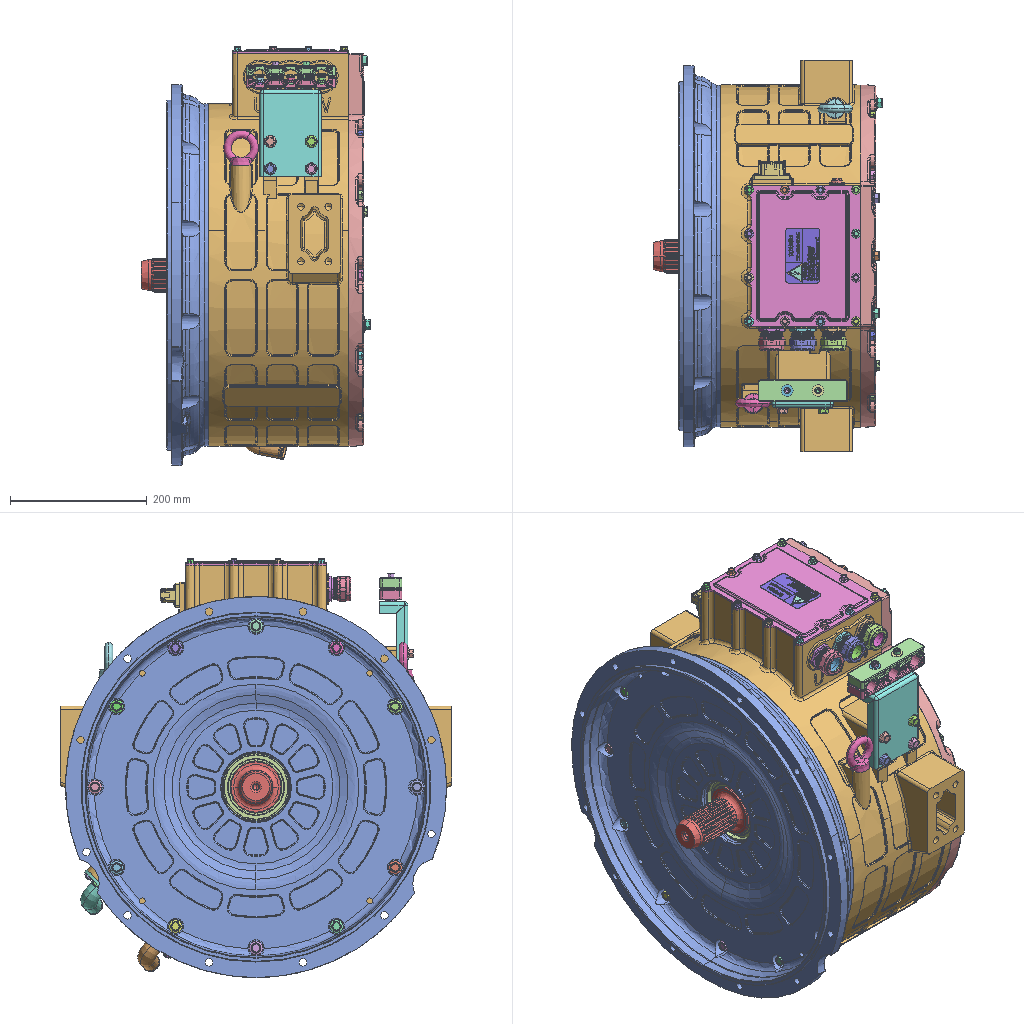Assembly | SolidWorks | 132 different items | 132 placed | box 335 x 572 x 612 mm
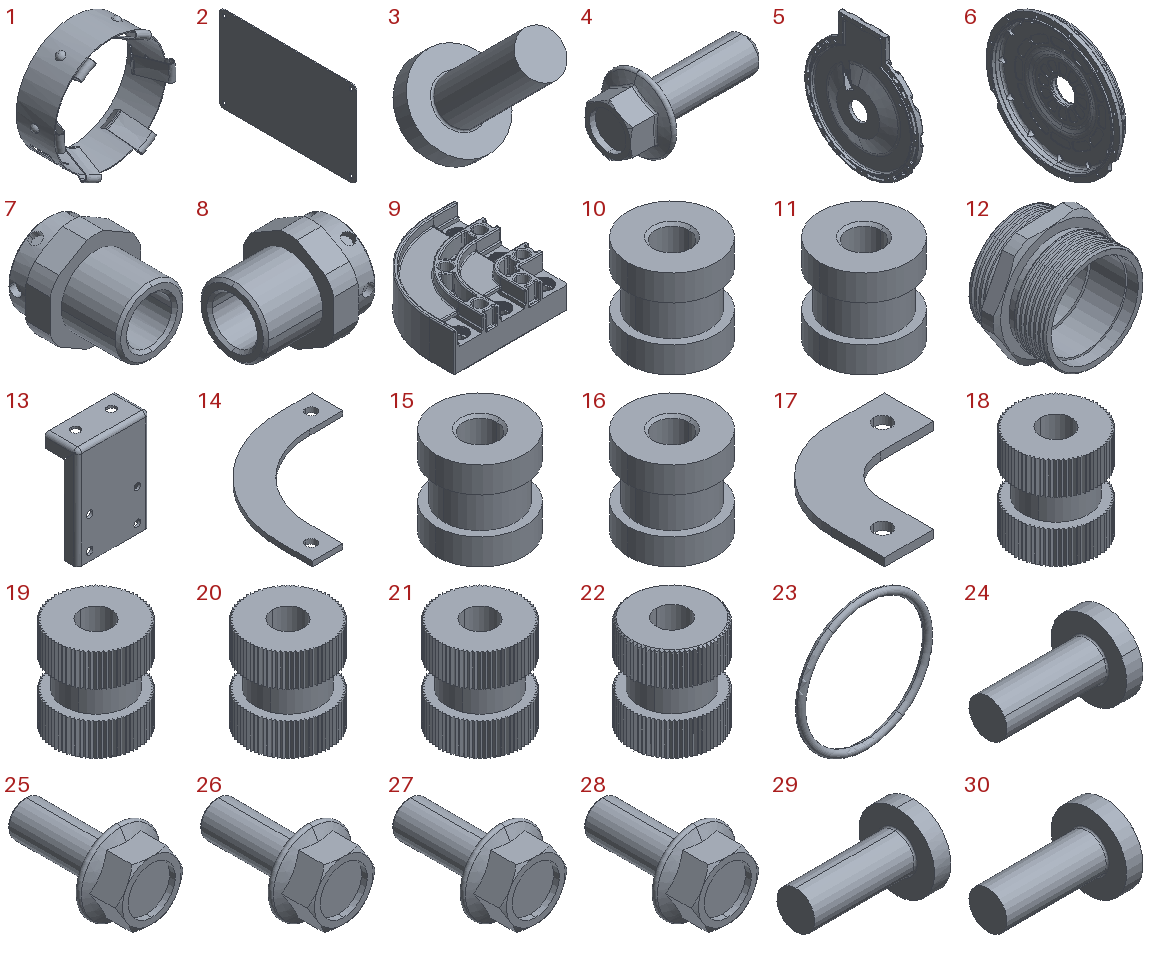Parts list (item | quantity | size | volume | features):
1 | x1 | 28 x 11 x 26.6 mm | 215.957 mm3 | features BaseBody 1
2 | x1 | - | 3306 mm3 | features BaseBody 1
3 | x1 | 12 x 19.516 x 19.516 mm | 825.398 mm3 | features BaseBody 1
4 | x1 | 39.7 x 20.8 x 20.8 mm | 3844 mm3 | features BaseBody 1
5 | x1 | 38.5 x 500 x 573.5 mm | 2957583 mm3 | features BaseBody 1
6 | x1 | 70 x 556.6 x 556.6 mm | 4634291 mm3 | features BaseBody 1
7 | x1 | 16 x 18.5 x 17 mm | 1862 mm3 | features BaseBody 1
8 | x1 | 18.5 x 16 x 17 mm | 1862 mm3 | features BaseBody 1
9 | x1 | 120 x 120 x 40 mm | 221994 mm3 | features BaseBody 1
10 | x1 | 17 x 17 x 17 mm | 2778 mm3 | features BaseBody 1
11 | x1 | 17 x 17 x 17 mm | 2778 mm3 | features BaseBody 1
12 | x1 | 39 x 25 x 36.772 mm | 7027 mm3 | features BaseBody 1
13 | x1 | 90 x 41 x 127.2 mm | 53821 mm3 | features BaseBody 1
14 | x1 | 115 x 115 x 4 mm | 16149 mm3 | features BaseBody 1
15 | x1 | 17 x 17 x 17 mm | 2778 mm3 | features BaseBody 1
16 | x1 | 17 x 17 x 17 mm | 2778 mm3 | features BaseBody 1
17 | x1 | 70 x 70 x 4 mm | 9364 mm3 | features BaseBody 1
18 | x1 | 18.005 x 18.005 x 20 mm | 3580 mm3 | features BaseBody 1
19 | x1 | 18.005 x 18.005 x 20 mm | 3580 mm3 | features BaseBody 1
20 | x1 | 18.005 x 18.005 x 20 mm | 3580 mm3 | features BaseBody 1
21 | x1 | 18.005 x 18.005 x 20 mm | 3580 mm3 | features BaseBody 1
22 | x1 | 18.005 x 18.005 x 20 mm | 3583 mm3 | features BaseBody 1
23 | x1 | 33.8 x 1.8 x 33.8 mm | 255.82 mm3 | features BaseBody 1
24 | x1 | 20.395 x 12 x 12 mm | 825.398 mm3 | features BaseBody 1
25 | x1 | 18 x 28.1 x 18 mm | 2194 mm3 | features BaseBody 1
26 | x1 | 18 x 28.1 x 18 mm | 2194 mm3 | features BaseBody 1
27 | x1 | 18 x 28.1 x 18 mm | 2194 mm3 | features BaseBody 1
28 | x1 | 18 x 28.1 x 18 mm | 2194 mm3 | features BaseBody 1
29 | x1 | 20.395 x 12 x 12 mm | 825.398 mm3 | features BaseBody 1
30 | x1 | 20.395 x 12 x 12 mm | 825.398 mm3 | features BaseBody 1
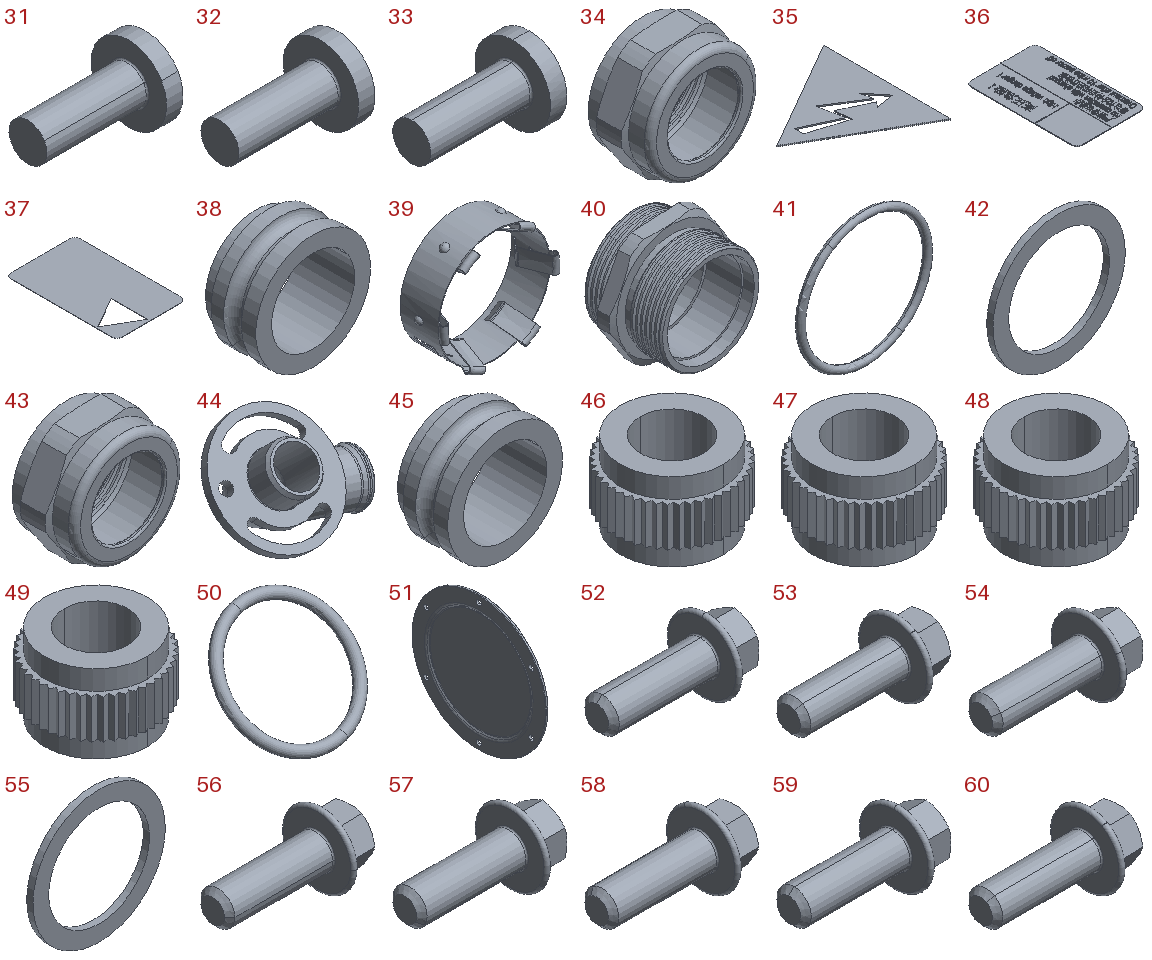31 | x1 | 20.395 x 12 x 12 mm | 825.398 mm3 | features BaseBody 1
32 | x1 | 20.395 x 12 x 12 mm | 825.398 mm3 | features BaseBody 1
33 | x1 | 20.395 x 12 x 12 mm | 825.398 mm3 | features BaseBody 1
34 | x1 | 39 x 20 x 36.772 mm | 4794 mm3 | features BaseBody 1
35 | x1 | 18.841 x 21.756 x 0.2 mm | 36.989 mm3 | features BaseBody 1
36 | x1 | 50 x 80 x 0.7 mm | 2057 mm3 | features BaseBody 1
37 | x1 | 50 x 80 x 0.2 mm | 739.101 mm3 | features BaseBody 1
38 | x1 | 32 x 16 x 32 mm | 4523 mm3 | features BaseBody 1
39 | x1 | 28 x 11 x 26.6 mm | 215.957 mm3 | features BaseBody 1
40 | x1 | 39 x 25 x 36.772 mm | 7027 mm3 | features BaseBody 1
41 | x1 | 33.8 x 1.8 x 33.8 mm | 255.82 mm3 | features BaseBody 1
42 | x1 | 31.8 x 1.5 x 31.8 mm | 501.398 mm3 | features BaseBody 1
43 | x1 | 39 x 20 x 36.772 mm | 4794 mm3 | features BaseBody 1
44 | x1 | 86.222 x 51.732 x 65.283 mm | 24499 mm3 | features BaseBody 1
45 | x1 | 32 x 16 x 32 mm | 4523 mm3 | features BaseBody 1
46 | x1 | 11.993 x 11.985 x 8 mm | 502.783 mm3 | features BaseBody 1
47 | x1 | 11.993 x 11.985 x 8 mm | 502.783 mm3 | features BaseBody 1
48 | x1 | 11.993 x 11.985 x 8 mm | 502.783 mm3 | features BaseBody 1
49 | x1 | 11.993 x 11.985 x 8 mm | 502.783 mm3 | features BaseBody 1
50 | x1 | 32.65 x 23.863 x 23.863 mm | 519.82 mm3 | features BaseBody 1
51 | x1 | 5 x 166 x 166 mm | 64748 mm3 | features BaseBody 1
52 | x1 | 39.7 x 20.8 x 20.8 mm | 3844 mm3 | features BaseBody 1
53 | x1 | 39.7 x 20.8 x 20.8 mm | 3844 mm3 | features BaseBody 1
54 | x1 | 39.7 x 20.8 x 20.8 mm | 3844 mm3 | features BaseBody 1
55 | x1 | 31.8 x 1.5 x 31.8 mm | 501.398 mm3 | features BaseBody 1
56 | x1 | 39.7 x 20.8 x 20.8 mm | 3844 mm3 | features BaseBody 1
57 | x1 | 39.7 x 20.8 x 20.8 mm | 3844 mm3 | features BaseBody 1
58 | x1 | 39.7 x 20.8 x 20.8 mm | 3844 mm3 | features BaseBody 1
59 | x1 | 39.7 x 20.8 x 20.8 mm | 3844 mm3 | features BaseBody 1
60 | x1 | 39.7 x 20.8 x 20.8 mm | 3844 mm3 | features BaseBody 1
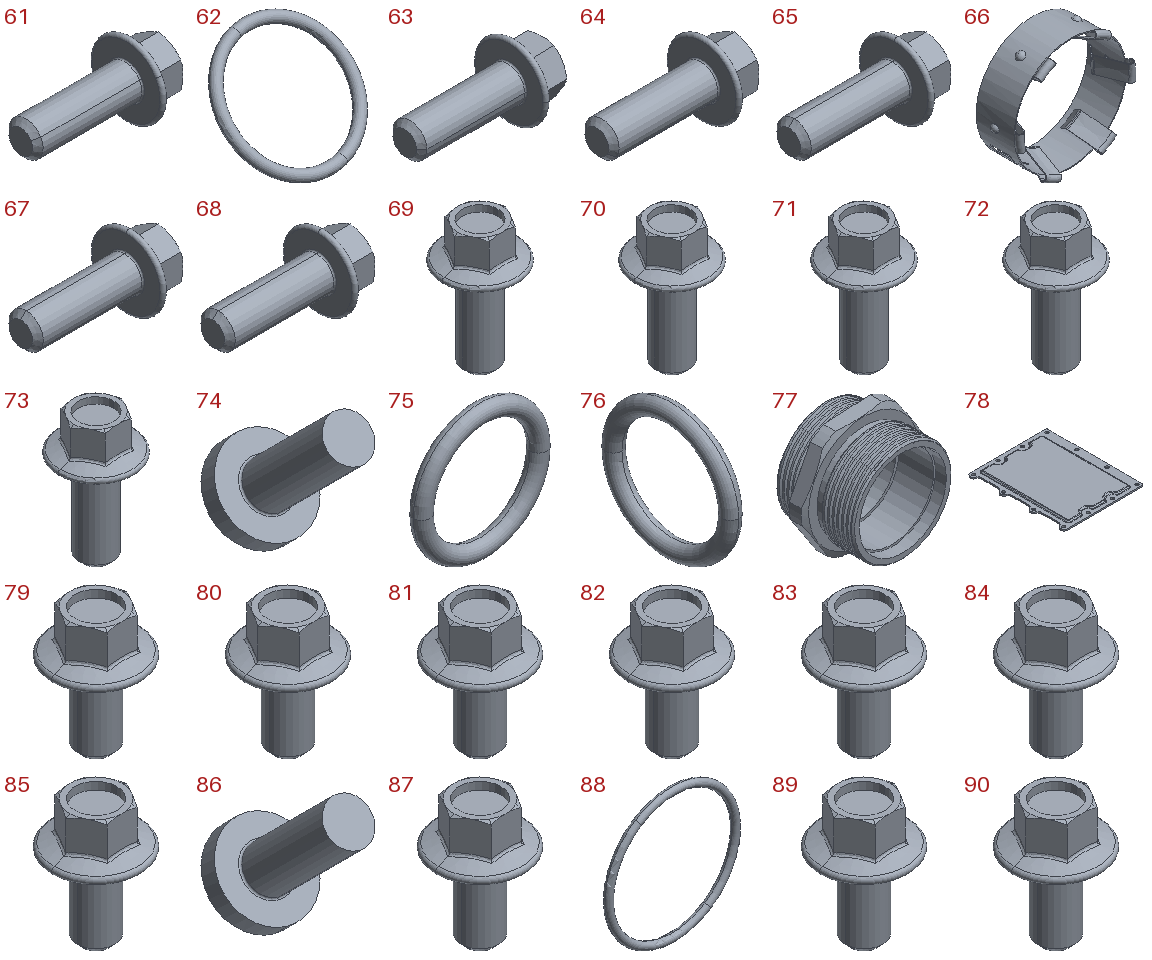61 | x1 | 39.7 x 20.8 x 20.8 mm | 3844 mm3 | features BaseBody 1
62 | x1 | 32.65 x 23.863 x 23.863 mm | 519.82 mm3 | features BaseBody 1
63 | x1 | 39.7 x 20.8 x 20.8 mm | 3844 mm3 | features BaseBody 1
64 | x1 | 39.7 x 20.8 x 20.8 mm | 3844 mm3 | features BaseBody 1
65 | x1 | 39.7 x 20.8 x 20.8 mm | 3844 mm3 | features BaseBody 1
66 | x1 | 28 x 11 x 26.6 mm | 215.957 mm3 | features BaseBody 1
67 | x1 | 39.7 x 20.8 x 20.8 mm | 3844 mm3 | features BaseBody 1
68 | x1 | 39.7 x 20.8 x 20.8 mm | 3844 mm3 | features BaseBody 1
69 | x1 | 17 x 17 x 28.5 mm | 1813 mm3 | features BaseBody 1
70 | x1 | 17 x 17 x 28.5 mm | 1813 mm3 | features BaseBody 1
71 | x1 | 17 x 17 x 28.5 mm | 1813 mm3 | features BaseBody 1
72 | x1 | 17 x 17 x 28.5 mm | 1813 mm3 | features BaseBody 1
73 | x1 | 17 x 17 x 28.5 mm | 1813 mm3 | features BaseBody 1
74 | x1 | 12 x 19.516 x 19.516 mm | 825.398 mm3 | features BaseBody 1
75 | x1 | 16 x 2 x 16 mm | 138.174 mm3 | features BaseBody 1
76 | x1 | 2 x 16 x 16 mm | 138.174 mm3 | features BaseBody 1
77 | x1 | 39 x 25 x 36.772 mm | 7027 mm3 | features BaseBody 1
78 | x1 | 170 x 206 x 6 mm | 103348 mm3 | features BaseBody 1
79 | x1 | 13.6 x 13.6 x 18.9 mm | 775.835 mm3 | features BaseBody 1
80 | x1 | 13.6 x 13.6 x 18.9 mm | 775.834 mm3 | features BaseBody 1
81 | x1 | 13.6 x 13.6 x 18.9 mm | 775.835 mm3 | features BaseBody 1
82 | x1 | 13.6 x 13.6 x 18.9 mm | 775.835 mm3 | features BaseBody 1
83 | x1 | 13.6 x 13.6 x 18.9 mm | 775.835 mm3 | features BaseBody 1
84 | x1 | 13.6 x 13.6 x 18.9 mm | 775.835 mm3 | features BaseBody 1
85 | x1 | 13.6 x 13.6 x 18.9 mm | 775.835 mm3 | features BaseBody 1
86 | x1 | 12 x 19.516 x 19.516 mm | 825.398 mm3 | features BaseBody 1
87 | x1 | 13.6 x 13.6 x 18.9 mm | 775.834 mm3 | features BaseBody 1
88 | x1 | 33.8 x 1.8 x 33.8 mm | 255.82 mm3 | features BaseBody 1
89 | x1 | 13.6 x 13.6 x 18.9 mm | 775.835 mm3 | features BaseBody 1
90 | x1 | 13.6 x 13.6 x 18.9 mm | 775.835 mm3 | features BaseBody 1
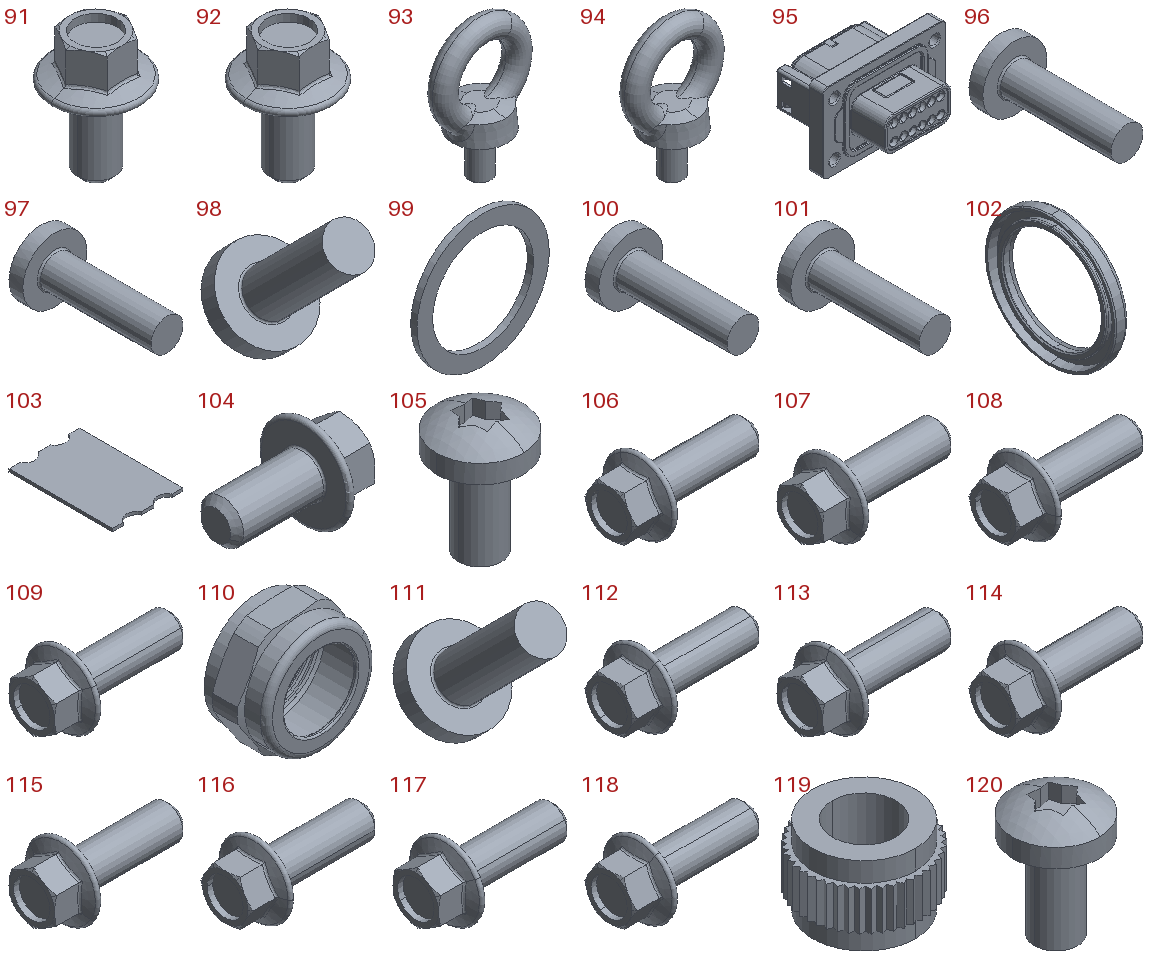91 | x1 | 13.6 x 13.6 x 18.9 mm | 775.835 mm3 | features BaseBody 1
92 | x1 | 13.6 x 13.6 x 18.9 mm | 775.835 mm3 | features BaseBody 1
93 | x1 | 51.2 x 29.1 x 73.6 mm | 20260 mm3 | features BaseBody 1
94 | x1 | 51.2 x 29.1 x 73.6 mm | 20260 mm3 | features BaseBody 1
95 | x1 | 55.12 x 43.688 x 35.56 mm | 26198 mm3 | features BaseBody 1
96 | x1 | 8 x 16.943 x 8 mm | 285.559 mm3 | features BaseBody 1
97 | x1 | 8 x 16.943 x 8 mm | 285.559 mm3 | features BaseBody 1
98 | x1 | 12 x 19.516 x 19.516 mm | 825.398 mm3 | features BaseBody 1
99 | x1 | 31.8 x 1.5 x 31.8 mm | 501.398 mm3 | features BaseBody 1
100 | x1 | 8 x 16.943 x 8 mm | 285.559 mm3 | features BaseBody 1
101 | x1 | 8 x 16.943 x 8 mm | 285.559 mm3 | features BaseBody 1
102 | x1 | 10 x 100 x 100 mm | 19515 mm3 | features BaseBody 1
103 | x1 | 120 x 176 x 5 mm | 101377 mm3 | features BaseBody 1
104 | x1 | 29.7 x 20.8 x 20.8 mm | 3100 mm3 | features BaseBody 1
105 | x1 | 8 x 8 x 10.943 mm | 210.161 mm3 | features BaseBody 1
106 | x1 | 39.7 x 20.8 x 20.8 mm | 3844 mm3 | features BaseBody 1
107 | x1 | 39.7 x 20.8 x 20.8 mm | 3844 mm3 | features BaseBody 1
108 | x1 | 39.7 x 20.8 x 20.8 mm | 3844 mm3 | features BaseBody 1
109 | x1 | 39.7 x 20.8 x 20.8 mm | 3844 mm3 | features BaseBody 1
110 | x1 | 39 x 20 x 36.772 mm | 4794 mm3 | features BaseBody 1
111 | x1 | 12 x 19.516 x 19.516 mm | 825.398 mm3 | features BaseBody 1
112 | x1 | 39.7 x 20.8 x 20.8 mm | 3844 mm3 | features BaseBody 1
113 | x1 | 39.7 x 20.8 x 20.8 mm | 3844 mm3 | features BaseBody 1
114 | x1 | 39.7 x 20.8 x 20.8 mm | 3844 mm3 | features BaseBody 1
115 | x1 | 39.7 x 20.8 x 20.8 mm | 3844 mm3 | features BaseBody 1
116 | x1 | 39.7 x 20.8 x 20.8 mm | 3844 mm3 | features BaseBody 1
117 | x1 | 39.7 x 20.8 x 20.8 mm | 3844 mm3 | features BaseBody 1
118 | x1 | 39.7 x 20.8 x 20.8 mm | 3844 mm3 | features BaseBody 1
119 | x1 | 11.993 x 11.985 x 8 mm | 502.783 mm3 | features BaseBody 1
120 | x1 | 8 x 8 x 10.943 mm | 210.161 mm3 | features BaseBody 1
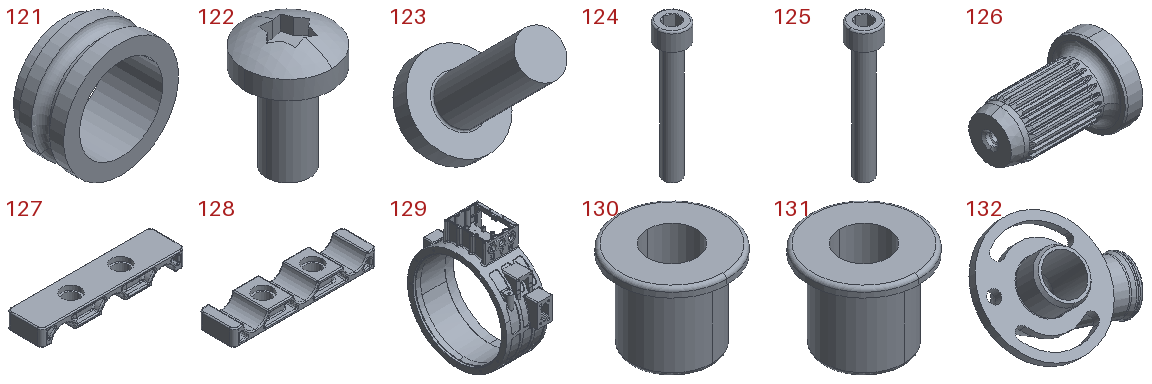121 | x1 | 32 x 16 x 32 mm | 4523 mm3 | features BaseBody 1
122 | x1 | 8 x 8 x 10.943 mm | 210.161 mm3 | features BaseBody 1
123 | x1 | 12 x 19.516 x 19.516 mm | 825.398 mm3 | features BaseBody 1
124 | x1 | 10 x 10 x 46 mm | 1433 mm3 | features BaseBody 1
125 | x1 | 10 x 10 x 46 mm | 1433 mm3 | features BaseBody 1
126 | x1 | 107 x 75 x 75 mm | 230700 mm3 | features BaseBody 1
127 | x1 | 130 x 32 x 15 mm | 34645 mm3 | features BaseBody 1
128 | x1 | 130 x 32 x 15 mm | 34645 mm3 | features BaseBody 1
129 | x1 | 205 x 571.5 x 574 mm | 7765718 mm3 | features BaseBody 1
130 | x1 | 15 x 15 x 12 mm | 798.307 mm3 | features BaseBody 1
131 | x1 | 15 x 15 x 12 mm | 798.307 mm3 | features BaseBody 1
132 | x1 | 86.222 x 51.732 x 65.283 mm | 24499 mm3 | features BaseBody 1